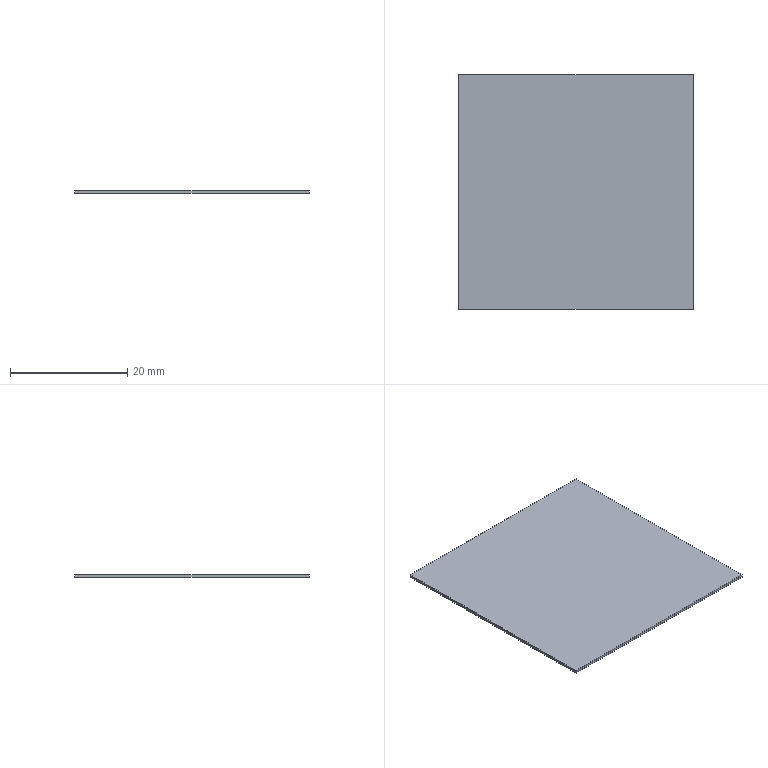Part | SolidWorks | features BaseBody 1 | 1 solid | 6 faces | box 40 x 40 x 0.5 mm | volume 800 mm3 | plane 6
STEP:
#1=CARTESIAN_POINT('',(-20.,22.,3.));
#2=VERTEX_POINT('',#1);
#3=CARTESIAN_POINT('',(-20.,-18.,3.));
#4=VERTEX_POINT('',#3);
#5=CARTESIAN_POINT('',(-20.,22.,3.));
#6=DIRECTION('',(0.,-1.,0.));
#7=VECTOR('',#6,1000.);
#8=LINE('',#5,#7);
#9=EDGE_CURVE('',#2,#4,#8,.T.);
#10=ORIENTED_EDGE('',*,*,#9,.T.);
#11=CARTESIAN_POINT('',(-20.,-18.,3.5));
#12=VERTEX_POINT('',#11);
#13=CARTESIAN_POINT('',(-20.,-18.,3.5));
#14=DIRECTION('',(0.,0.,-1.));
#15=VECTOR('',#14,1000.);
#16=LINE('',#13,#15);
#17=EDGE_CURVE('',#12,#4,#16,.T.);
#18=ORIENTED_EDGE('',*,*,#17,.F.);
#19=CARTESIAN_POINT('',(-20.,22.,3.5));
#20=VERTEX_POINT('',#19);
#21=CARTESIAN_POINT('',(-20.,22.,3.5));
#22=DIRECTION('',(0.,-1.,0.));
#23=VECTOR('',#22,1000.);
#24=LINE('',#21,#23);
#25=EDGE_CURVE('',#20,#12,#24,.T.);
#26=ORIENTED_EDGE('',*,*,#25,.F.);
#27=CARTESIAN_POINT('',(-20.,22.,3.5));
#28=DIRECTION('',(0.,0.,-1.));
#29=VECTOR('',#28,1000.);
#30=LINE('',#27,#29);
#31=EDGE_CURVE('',#20,#2,#30,.T.);
#32=ORIENTED_EDGE('',*,*,#31,.T.);
#33=EDGE_LOOP('',(#10,#18,#26,#32));
#34=FACE_OUTER_BOUND('',#33,.T.);
#35=CARTESIAN_POINT('',(-20.,22.,3.5));
#36=DIRECTION('',(1.,0.,0.));
#37=DIRECTION('',(0.,0.,-1.));
#38=AXIS2_PLACEMENT_3D('',#35,#36,#37);
#39=PLANE('',#38);
#40=ADVANCED_FACE('',(#34),#39,.F.);
#41=CARTESIAN_POINT('',(20.,-18.,3.));
#42=VERTEX_POINT('',#41);
#43=CARTESIAN_POINT('',(-20.,-18.,3.));
#44=DIRECTION('',(1.,0.,0.));
#45=VECTOR('',#44,1000.);
#46=LINE('',#43,#45);
#47=EDGE_CURVE('',#4,#42,#46,.T.);
#48=ORIENTED_EDGE('',*,*,#47,.T.);
#49=CARTESIAN_POINT('',(20.,-18.,3.5));
#50=VERTEX_POINT('',#49);
#51=CARTESIAN_POINT('',(20.,-18.,3.5));
#52=DIRECTION('',(0.,0.,-1.));
#53=VECTOR('',#52,1000.);
#54=LINE('',#51,#53);
#55=EDGE_CURVE('',#50,#42,#54,.T.);
#56=ORIENTED_EDGE('',*,*,#55,.F.);
#57=CARTESIAN_POINT('',(-20.,-18.,3.5));
#58=DIRECTION('',(1.,0.,0.));
#59=VECTOR('',#58,1000.);
#60=LINE('',#57,#59);
#61=EDGE_CURVE('',#12,#50,#60,.T.);
#62=ORIENTED_EDGE('',*,*,#61,.F.);
#63=ORIENTED_EDGE('',*,*,#17,.T.);
#64=EDGE_LOOP('',(#48,#56,#62,#63));
#65=FACE_OUTER_BOUND('',#64,.T.);
#66=CARTESIAN_POINT('',(-20.,-18.,3.5));
#67=DIRECTION('',(0.,1.,0.));
#68=DIRECTION('',(-1.,0.,0.));
#69=AXIS2_PLACEMENT_3D('',#66,#67,#68);
#70=PLANE('',#69);
#71=ADVANCED_FACE('',(#65),#70,.F.);
#72=CARTESIAN_POINT('',(20.,22.,3.));
#73=VERTEX_POINT('',#72);
#74=CARTESIAN_POINT('',(20.,-18.,3.));
#75=DIRECTION('',(0.,1.,0.));
#76=VECTOR('',#75,1000.);
#77=LINE('',#74,#76);
#78=EDGE_CURVE('',#42,#73,#77,.T.);
#79=ORIENTED_EDGE('',*,*,#78,.T.);
#80=CARTESIAN_POINT('',(20.,22.,3.5));
#81=VERTEX_POINT('',#80);
#82=CARTESIAN_POINT('',(20.,22.,3.5));
#83=DIRECTION('',(0.,0.,-1.));
#84=VECTOR('',#83,1000.);
#85=LINE('',#82,#84);
#86=EDGE_CURVE('',#81,#73,#85,.T.);
#87=ORIENTED_EDGE('',*,*,#86,.F.);
#88=CARTESIAN_POINT('',(20.,-18.,3.5));
#89=DIRECTION('',(0.,1.,0.));
#90=VECTOR('',#89,1000.);
#91=LINE('',#88,#90);
#92=EDGE_CURVE('',#50,#81,#91,.T.);
#93=ORIENTED_EDGE('',*,*,#92,.F.);
#94=ORIENTED_EDGE('',*,*,#55,.T.);
#95=EDGE_LOOP('',(#79,#87,#93,#94));
#96=FACE_OUTER_BOUND('',#95,.T.);
#97=CARTESIAN_POINT('',(20.,-18.,3.5));
#98=DIRECTION('',(-1.,0.,0.));
#99=DIRECTION('',(0.,-1.,0.));
#100=AXIS2_PLACEMENT_3D('',#97,#98,#99);
#101=PLANE('',#100);
#102=ADVANCED_FACE('',(#96),#101,.F.);
#103=CARTESIAN_POINT('',(20.,22.,3.));
#104=DIRECTION('',(-1.,0.,0.));
#105=VECTOR('',#104,1000.);
#106=LINE('',#103,#105);
#107=EDGE_CURVE('',#73,#2,#106,.T.);
#108=ORIENTED_EDGE('',*,*,#107,.T.);
#109=ORIENTED_EDGE('',*,*,#31,.F.);
#110=CARTESIAN_POINT('',(20.,22.,3.5));
#111=DIRECTION('',(-1.,0.,0.));
#112=VECTOR('',#111,1000.);
#113=LINE('',#110,#112);
#114=EDGE_CURVE('',#81,#20,#113,.T.);
#115=ORIENTED_EDGE('',*,*,#114,.F.);
#116=ORIENTED_EDGE('',*,*,#86,.T.);
#117=EDGE_LOOP('',(#108,#109,#115,#116));
#118=FACE_OUTER_BOUND('',#117,.T.);
#119=CARTESIAN_POINT('',(20.,22.,3.5));
#120=DIRECTION('',(0.,-1.,0.));
#121=DIRECTION('',(0.,0.,-1.));
#122=AXIS2_PLACEMENT_3D('',#119,#120,#121);
#123=PLANE('',#122);
#124=ADVANCED_FACE('',(#118),#123,.F.);
#125=ORIENTED_EDGE('',*,*,#25,.T.);
#126=ORIENTED_EDGE('',*,*,#61,.T.);
#127=ORIENTED_EDGE('',*,*,#92,.T.);
#128=ORIENTED_EDGE('',*,*,#114,.T.);
#129=EDGE_LOOP('',(#125,#126,#127,#128));
#130=FACE_OUTER_BOUND('',#129,.T.);
#131=CARTESIAN_POINT('',(0.,0.,3.5));
#132=DIRECTION('',(0.,0.,1.));
#133=DIRECTION('',(1.,0.,0.));
#134=AXIS2_PLACEMENT_3D('',#131,#132,#133);
#135=PLANE('',#134);
#136=ADVANCED_FACE('',(#130),#135,.T.);
#137=ORIENTED_EDGE('',*,*,#9,.F.);
#138=ORIENTED_EDGE('',*,*,#107,.F.);
#139=ORIENTED_EDGE('',*,*,#78,.F.);
#140=ORIENTED_EDGE('',*,*,#47,.F.);
#141=EDGE_LOOP('',(#137,#138,#139,#140));
#142=FACE_OUTER_BOUND('',#141,.T.);
#143=CARTESIAN_POINT('',(0.,0.,3.));
#144=DIRECTION('',(0.,0.,1.));
#145=DIRECTION('',(1.,0.,0.));
#146=AXIS2_PLACEMENT_3D('',#143,#144,#145);
#147=PLANE('',#146);
#148=ADVANCED_FACE('',(#142),#147,.F.);
#149=CLOSED_SHELL('',(#40,#71,#102,#124,#136,#148));
#150=MANIFOLD_SOLID_BREP('',#149);
#151=CARTESIAN_POINT('',(0.,0.,0.));
#152=DIRECTION('',(0.,0.,1.));
#153=DIRECTION('',(1.,0.,0.));
#154=AXIS2_PLACEMENT_3D('',#151,#152,#153);
#155=(LENGTH_UNIT()NAMED_UNIT(*)SI_UNIT(.MILLI.,.METRE.));
#156=UNCERTAINTY_MEASURE_WITH_UNIT(LENGTH_MEASURE(0.00001),#155,'','');
#157=(NAMED_UNIT(*)PLANE_ANGLE_UNIT()SI_UNIT($,.RADIAN.));
#158=(NAMED_UNIT(*)SI_UNIT($,.STERADIAN.)SOLID_ANGLE_UNIT());
#159=(GEOMETRIC_REPRESENTATION_CONTEXT(3)GLOBAL_UNCERTAINTY_ASSIGNED_CONTEXT((#156))GLOBAL_UNIT_ASSIGNED_CONTEXT((#155,#157,#158))REPRESENTATION_CONTEXT('',''));
#160=ADVANCED_BREP_SHAPE_REPRESENTATION('',(#150,#154),#159);